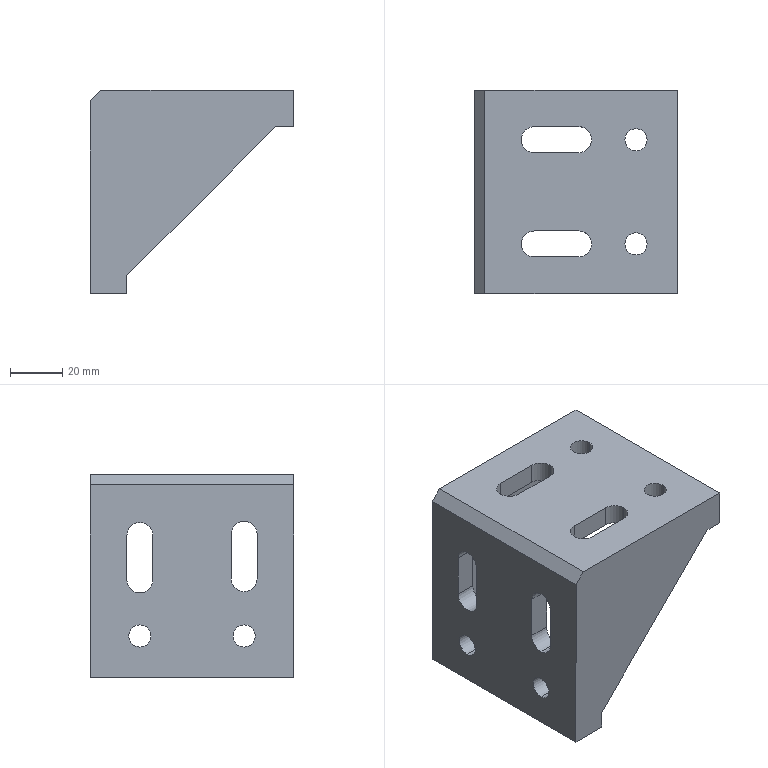Part | SolidWorks | features ICE 11, HoleWzd 2, Chamfer 1, Extrusion 1 | 1 solid | 45 faces | box 78 x 78 x 78 mm | volume 101387 mm3 | plane 25 | cylinder 20 | commonest cylinder face diameters 10 x12 8.5 x8
STEP:
#1=CARTESIAN_POINT('',(24.019,19.,55.578));
#2=VERTEX_POINT('',#1);
#3=CARTESIAN_POINT('',(32.519,19.,55.578));
#4=VERTEX_POINT('',#3);
#5=CARTESIAN_POINT('',(28.269,19.,55.578));
#6=DIRECTION('',(0.,0.,1.));
#7=DIRECTION('',(1.,0.,0.));
#8=AXIS2_PLACEMENT_3D('',#5,#6,#7);
#9=CIRCLE('',#8,4.25);
#10=EDGE_CURVE('',#2,#4,#9,.T.);
#11=ORIENTED_EDGE('',*,*,#10,.F.);
#12=CARTESIAN_POINT('',(24.019,19.,63.578));
#13=VERTEX_POINT('',#12);
#14=CARTESIAN_POINT('',(24.019,19.,63.578));
#15=DIRECTION('',(0.,0.,1.));
#16=VECTOR('',#15,1000.);
#17=LINE('',#14,#16);
#18=EDGE_CURVE('',#2,#13,#17,.T.);
#19=ORIENTED_EDGE('',*,*,#18,.T.);
#20=CARTESIAN_POINT('',(32.519,19.,63.578));
#21=VERTEX_POINT('',#20);
#22=CARTESIAN_POINT('',(28.269,19.,63.578));
#23=DIRECTION('',(0.,0.,1.));
#24=DIRECTION('',(1.,0.,0.));
#25=AXIS2_PLACEMENT_3D('',#22,#23,#24);
#26=CIRCLE('',#25,4.25);
#27=EDGE_CURVE('',#13,#21,#26,.T.);
#28=ORIENTED_EDGE('',*,*,#27,.T.);
#29=CARTESIAN_POINT('',(32.519,19.,63.578));
#30=DIRECTION('',(0.,0.,1.));
#31=VECTOR('',#30,1000.);
#32=LINE('',#29,#31);
#33=EDGE_CURVE('',#4,#21,#32,.T.);
#34=ORIENTED_EDGE('',*,*,#33,.F.);
#35=EDGE_LOOP('',(#11,#19,#28,#34));
#36=FACE_OUTER_BOUND('',#35,.T.);
#37=CARTESIAN_POINT('',(28.269,19.,63.578));
#38=DIRECTION('',(0.,0.,1.));
#39=DIRECTION('',(1.,0.,0.));
#40=AXIS2_PLACEMENT_3D('',#37,#38,#39);
#41=CYLINDRICAL_SURFACE('',#40,4.25);
#42=ADVANCED_FACE('',(#36),#41,.F.);
#43=CARTESIAN_POINT('',(24.019,59.,55.578));
#44=VERTEX_POINT('',#43);
#45=CARTESIAN_POINT('',(32.519,59.,55.578));
#46=VERTEX_POINT('',#45);
#47=CARTESIAN_POINT('',(28.269,59.,55.578));
#48=DIRECTION('',(0.,0.,1.));
#49=DIRECTION('',(1.,0.,0.));
#50=AXIS2_PLACEMENT_3D('',#47,#48,#49);
#51=CIRCLE('',#50,4.25);
#52=EDGE_CURVE('',#44,#46,#51,.T.);
#53=ORIENTED_EDGE('',*,*,#52,.F.);
#54=CARTESIAN_POINT('',(24.019,59.,63.578));
#55=VERTEX_POINT('',#54);
#56=CARTESIAN_POINT('',(24.019,59.,63.578));
#57=DIRECTION('',(0.,0.,1.));
#58=VECTOR('',#57,1000.);
#59=LINE('',#56,#58);
#60=EDGE_CURVE('',#44,#55,#59,.T.);
#61=ORIENTED_EDGE('',*,*,#60,.T.);
#62=CARTESIAN_POINT('',(32.519,59.,63.578));
#63=VERTEX_POINT('',#62);
#64=CARTESIAN_POINT('',(28.269,59.,63.578));
#65=DIRECTION('',(0.,0.,1.));
#66=DIRECTION('',(1.,0.,0.));
#67=AXIS2_PLACEMENT_3D('',#64,#65,#66);
#68=CIRCLE('',#67,4.25);
#69=EDGE_CURVE('',#55,#63,#68,.T.);
#70=ORIENTED_EDGE('',*,*,#69,.T.);
#71=CARTESIAN_POINT('',(32.519,59.,63.578));
#72=DIRECTION('',(0.,0.,1.));
#73=VECTOR('',#72,1000.);
#74=LINE('',#71,#73);
#75=EDGE_CURVE('',#46,#63,#74,.T.);
#76=ORIENTED_EDGE('',*,*,#75,.F.);
#77=EDGE_LOOP('',(#53,#61,#70,#76));
#78=FACE_OUTER_BOUND('',#77,.T.);
#79=CARTESIAN_POINT('',(28.269,59.,63.578));
#80=DIRECTION('',(0.,0.,1.));
#81=DIRECTION('',(1.,0.,0.));
#82=AXIS2_PLACEMENT_3D('',#79,#80,#81);
#83=CYLINDRICAL_SURFACE('',#82,4.25);
#84=ADVANCED_FACE('',(#78),#83,.F.);
#85=CARTESIAN_POINT('',(-25.731,59.,-2.672));
#86=VERTEX_POINT('',#85);
#87=CARTESIAN_POINT('',(-25.731,59.,5.828));
#88=VERTEX_POINT('',#87);
#89=CARTESIAN_POINT('',(-25.731,59.,1.578));
#90=DIRECTION('',(-1.,0.,0.));
#91=DIRECTION('',(0.,0.,1.));
#92=AXIS2_PLACEMENT_3D('',#89,#90,#91);
#93=CIRCLE('',#92,4.25);
#94=EDGE_CURVE('',#86,#88,#93,.T.);
#95=ORIENTED_EDGE('',*,*,#94,.F.);
#96=CARTESIAN_POINT('',(-33.731,59.,-2.672));
#97=VERTEX_POINT('',#96);
#98=CARTESIAN_POINT('',(-33.731,59.,-2.672));
#99=DIRECTION('',(-1.,0.,0.));
#100=VECTOR('',#99,1000.);
#101=LINE('',#98,#100);
#102=EDGE_CURVE('',#86,#97,#101,.T.);
#103=ORIENTED_EDGE('',*,*,#102,.T.);
#104=CARTESIAN_POINT('',(-33.731,59.,5.828));
#105=VERTEX_POINT('',#104);
#106=CARTESIAN_POINT('',(-33.731,59.,1.578));
#107=DIRECTION('',(-1.,0.,0.));
#108=DIRECTION('',(0.,0.,1.));
#109=AXIS2_PLACEMENT_3D('',#106,#107,#108);
#110=CIRCLE('',#109,4.25);
#111=EDGE_CURVE('',#97,#105,#110,.T.);
#112=ORIENTED_EDGE('',*,*,#111,.T.);
#113=CARTESIAN_POINT('',(-33.731,59.,5.828));
#114=DIRECTION('',(-1.,0.,0.));
#115=VECTOR('',#114,1000.);
#116=LINE('',#113,#115);
#117=EDGE_CURVE('',#88,#105,#116,.T.);
#118=ORIENTED_EDGE('',*,*,#117,.F.);
#119=EDGE_LOOP('',(#95,#103,#112,#118));
#120=FACE_OUTER_BOUND('',#119,.T.);
#121=CARTESIAN_POINT('',(-33.731,59.,1.578));
#122=DIRECTION('',(-1.,0.,0.));
#123=DIRECTION('',(0.,0.,1.));
#124=AXIS2_PLACEMENT_3D('',#121,#122,#123);
#125=CYLINDRICAL_SURFACE('',#124,4.25);
#126=ADVANCED_FACE('',(#120),#125,.F.);
#127=CARTESIAN_POINT('',(-25.731,19.,-2.672));
#128=VERTEX_POINT('',#127);
#129=CARTESIAN_POINT('',(-25.731,19.,5.828));
#130=VERTEX_POINT('',#129);
#131=CARTESIAN_POINT('',(-25.731,19.,1.578));
#132=DIRECTION('',(-1.,0.,0.));
#133=DIRECTION('',(0.,0.,1.));
#134=AXIS2_PLACEMENT_3D('',#131,#132,#133);
#135=CIRCLE('',#134,4.25);
#136=EDGE_CURVE('',#128,#130,#135,.T.);
#137=ORIENTED_EDGE('',*,*,#136,.F.);
#138=CARTESIAN_POINT('',(-33.731,19.,-2.672));
#139=VERTEX_POINT('',#138);
#140=CARTESIAN_POINT('',(-33.731,19.,-2.672));
#141=DIRECTION('',(-1.,0.,0.));
#142=VECTOR('',#141,1000.);
#143=LINE('',#140,#142);
#144=EDGE_CURVE('',#128,#139,#143,.T.);
#145=ORIENTED_EDGE('',*,*,#144,.T.);
#146=CARTESIAN_POINT('',(-33.731,19.,5.828));
#147=VERTEX_POINT('',#146);
#148=CARTESIAN_POINT('',(-33.731,19.,1.578));
#149=DIRECTION('',(-1.,0.,0.));
#150=DIRECTION('',(0.,0.,1.));
#151=AXIS2_PLACEMENT_3D('',#148,#149,#150);
#152=CIRCLE('',#151,4.25);
#153=EDGE_CURVE('',#139,#147,#152,.T.);
#154=ORIENTED_EDGE('',*,*,#153,.T.);
#155=CARTESIAN_POINT('',(-33.731,19.,5.828));
#156=DIRECTION('',(-1.,0.,0.));
#157=VECTOR('',#156,1000.);
#158=LINE('',#155,#157);
#159=EDGE_CURVE('',#130,#147,#158,.T.);
#160=ORIENTED_EDGE('',*,*,#159,.F.);
#161=EDGE_LOOP('',(#137,#145,#154,#160));
#162=FACE_OUTER_BOUND('',#161,.T.);
#163=CARTESIAN_POINT('',(-33.731,19.,1.578));
#164=DIRECTION('',(-1.,0.,0.));
#165=DIRECTION('',(0.,0.,1.));
#166=AXIS2_PLACEMENT_3D('',#163,#164,#165);
#167=CYLINDRICAL_SURFACE('',#166,4.25);
#168=ADVANCED_FACE('',(#162),#167,.F.);
#169=CARTESIAN_POINT('',(-25.731,59.,45.078));
#170=VERTEX_POINT('',#169);
#171=CARTESIAN_POINT('',(-25.731,64.,40.078));
#172=VERTEX_POINT('',#171);
#173=CARTESIAN_POINT('',(-25.731,59.,40.078));
#174=DIRECTION('',(-1.,0.,0.));
#175=DIRECTION('',(0.,0.,1.));
#176=AXIS2_PLACEMENT_3D('',#173,#174,#175);
#177=CIRCLE('',#176,5.);
#178=EDGE_CURVE('',#170,#172,#177,.T.);
#179=ORIENTED_EDGE('',*,*,#178,.F.);
#180=CARTESIAN_POINT('',(-33.731,59.,45.078));
#181=VERTEX_POINT('',#180);
#182=CARTESIAN_POINT('',(44.269,59.,45.078));
#183=DIRECTION('',(-1.,0.,0.));
#184=VECTOR('',#183,1000.);
#185=LINE('',#182,#184);
#186=EDGE_CURVE('',#170,#181,#185,.T.);
#187=ORIENTED_EDGE('',*,*,#186,.T.);
#188=CARTESIAN_POINT('',(-33.731,64.,40.078));
#189=VERTEX_POINT('',#188);
#190=CARTESIAN_POINT('',(-33.731,59.,40.078));
#191=DIRECTION('',(-1.,0.,0.));
#192=DIRECTION('',(0.,0.,1.));
#193=AXIS2_PLACEMENT_3D('',#190,#191,#192);
#194=CIRCLE('',#193,5.);
#195=EDGE_CURVE('',#181,#189,#194,.T.);
#196=ORIENTED_EDGE('',*,*,#195,.T.);
#197=CARTESIAN_POINT('',(44.269,64.,40.078));
#198=DIRECTION('',(-1.,0.,0.));
#199=VECTOR('',#198,1000.);
#200=LINE('',#197,#199);
#201=EDGE_CURVE('',#172,#189,#200,.T.);
#202=ORIENTED_EDGE('',*,*,#201,.F.);
#203=EDGE_LOOP('',(#179,#187,#196,#202));
#204=FACE_OUTER_BOUND('',#203,.T.);
#205=CARTESIAN_POINT('',(44.269,59.,40.078));
#206=DIRECTION('',(-1.,0.,0.));
#207=DIRECTION('',(0.,0.,1.));
#208=AXIS2_PLACEMENT_3D('',#205,#206,#207);
#209=CYLINDRICAL_SURFACE('',#208,5.);
#210=ADVANCED_FACE('',(#204),#209,.F.);
#211=CARTESIAN_POINT('',(11.269,19.,55.578));
#212=VERTEX_POINT('',#211);
#213=CARTESIAN_POINT('',(6.269,24.,55.578));
#214=VERTEX_POINT('',#213);
#215=CARTESIAN_POINT('',(6.269,19.,55.578));
#216=DIRECTION('',(0.,0.,1.));
#217=DIRECTION('',(1.,0.,0.));
#218=AXIS2_PLACEMENT_3D('',#215,#216,#217);
#219=CIRCLE('',#218,5.);
#220=EDGE_CURVE('',#212,#214,#219,.T.);
#221=ORIENTED_EDGE('',*,*,#220,.F.);
#222=CARTESIAN_POINT('',(11.269,19.,63.578));
#223=VERTEX_POINT('',#222);
#224=CARTESIAN_POINT('',(11.269,19.,-14.422));
#225=DIRECTION('',(0.,0.,1.));
#226=VECTOR('',#225,1000.);
#227=LINE('',#224,#226);
#228=EDGE_CURVE('',#212,#223,#227,.T.);
#229=ORIENTED_EDGE('',*,*,#228,.T.);
#230=CARTESIAN_POINT('',(6.269,24.,63.578));
#231=VERTEX_POINT('',#230);
#232=CARTESIAN_POINT('',(6.269,19.,63.578));
#233=DIRECTION('',(0.,0.,1.));
#234=DIRECTION('',(1.,0.,0.));
#235=AXIS2_PLACEMENT_3D('',#232,#233,#234);
#236=CIRCLE('',#235,5.);
#237=EDGE_CURVE('',#223,#231,#236,.T.);
#238=ORIENTED_EDGE('',*,*,#237,.T.);
#239=CARTESIAN_POINT('',(6.269,24.,-14.422));
#240=DIRECTION('',(0.,0.,1.));
#241=VECTOR('',#240,1000.);
#242=LINE('',#239,#241);
#243=EDGE_CURVE('',#214,#231,#242,.T.);
#244=ORIENTED_EDGE('',*,*,#243,.F.);
#245=EDGE_LOOP('',(#221,#229,#238,#244));
#246=FACE_OUTER_BOUND('',#245,.T.);
#247=CARTESIAN_POINT('',(6.269,19.,-14.422));
#248=DIRECTION('',(0.,0.,1.));
#249=DIRECTION('',(1.,0.,0.));
#250=AXIS2_PLACEMENT_3D('',#247,#248,#249);
#251=CYLINDRICAL_SURFACE('',#250,5.);
#252=ADVANCED_FACE('',(#246),#251,.F.);
#253=CARTESIAN_POINT('',(11.269,59.,55.578));
#254=VERTEX_POINT('',#253);
#255=CARTESIAN_POINT('',(6.269,64.,55.578));
#256=VERTEX_POINT('',#255);
#257=CARTESIAN_POINT('',(6.269,59.,55.578));
#258=DIRECTION('',(0.,0.,1.));
#259=DIRECTION('',(1.,0.,0.));
#260=AXIS2_PLACEMENT_3D('',#257,#258,#259);
#261=CIRCLE('',#260,5.);
#262=EDGE_CURVE('',#254,#256,#261,.T.);
#263=ORIENTED_EDGE('',*,*,#262,.F.);
#264=CARTESIAN_POINT('',(11.269,59.,63.578));
#265=VERTEX_POINT('',#264);
#266=CARTESIAN_POINT('',(11.269,59.,-14.422));
#267=DIRECTION('',(0.,0.,1.));
#268=VECTOR('',#267,1000.);
#269=LINE('',#266,#268);
#270=EDGE_CURVE('',#254,#265,#269,.T.);
#271=ORIENTED_EDGE('',*,*,#270,.T.);
#272=CARTESIAN_POINT('',(6.269,64.,63.578));
#273=VERTEX_POINT('',#272);
#274=CARTESIAN_POINT('',(6.269,59.,63.578));
#275=DIRECTION('',(0.,0.,1.));
#276=DIRECTION('',(1.,0.,0.));
#277=AXIS2_PLACEMENT_3D('',#274,#275,#276);
#278=CIRCLE('',#277,5.);
#279=EDGE_CURVE('',#265,#273,#278,.T.);
#280=ORIENTED_EDGE('',*,*,#279,.T.);
#281=CARTESIAN_POINT('',(6.269,64.,-14.422));
#282=DIRECTION('',(0.,0.,1.));
#283=VECTOR('',#282,1000.);
#284=LINE('',#281,#283);
#285=EDGE_CURVE('',#256,#273,#284,.T.);
#286=ORIENTED_EDGE('',*,*,#285,.F.);
#287=EDGE_LOOP('',(#263,#271,#280,#286));
#288=FACE_OUTER_BOUND('',#287,.T.);
#289=CARTESIAN_POINT('',(6.269,59.,-14.422));
#290=DIRECTION('',(0.,0.,1.));
#291=DIRECTION('',(1.,0.,0.));
#292=AXIS2_PLACEMENT_3D('',#289,#290,#291);
#293=CYLINDRICAL_SURFACE('',#292,5.);
#294=ADVANCED_FACE('',(#288),#293,.F.);
#295=CARTESIAN_POINT('',(-33.731,19.,18.578));
#296=VERTEX_POINT('',#295);
#297=CARTESIAN_POINT('',(-33.731,24.,23.578));
#298=VERTEX_POINT('',#297);
#299=CARTESIAN_POINT('',(-33.731,19.,23.578));
#300=DIRECTION('',(1.,0.,0.));
#301=DIRECTION('',(0.,0.,-1.));
#302=AXIS2_PLACEMENT_3D('',#299,#300,#301);
#303=CIRCLE('',#302,5.);
#304=EDGE_CURVE('',#296,#298,#303,.T.);
#305=ORIENTED_EDGE('',*,*,#304,.F.);
#306=CARTESIAN_POINT('',(-25.731,19.,18.578));
#307=VERTEX_POINT('',#306);
#308=CARTESIAN_POINT('',(-33.731,19.,18.578));
#309=DIRECTION('',(1.,0.,0.));
#310=VECTOR('',#309,1000.);
#311=LINE('',#308,#310);
#312=EDGE_CURVE('',#296,#307,#311,.T.);
#313=ORIENTED_EDGE('',*,*,#312,.T.);
#314=CARTESIAN_POINT('',(-25.731,24.,23.578));
#315=VERTEX_POINT('',#314);
#316=CARTESIAN_POINT('',(-25.731,19.,23.578));
#317=DIRECTION('',(1.,0.,0.));
#318=DIRECTION('',(0.,0.,-1.));
#319=AXIS2_PLACEMENT_3D('',#316,#317,#318);
#320=CIRCLE('',#319,5.);
#321=EDGE_CURVE('',#307,#315,#320,.T.);
#322=ORIENTED_EDGE('',*,*,#321,.T.);
#323=CARTESIAN_POINT('',(-33.731,24.,23.578));
#324=DIRECTION('',(1.,0.,0.));
#325=VECTOR('',#324,1000.);
#326=LINE('',#323,#325);
#327=EDGE_CURVE('',#298,#315,#326,.T.);
#328=ORIENTED_EDGE('',*,*,#327,.F.);
#329=EDGE_LOOP('',(#305,#313,#322,#328));
#330=FACE_OUTER_BOUND('',#329,.T.);
#331=CARTESIAN_POINT('',(-33.731,19.,23.578));
#332=DIRECTION('',(1.,0.,0.));
#333=DIRECTION('',(0.,0.,-1.));
#334=AXIS2_PLACEMENT_3D('',#331,#332,#333);
#335=CYLINDRICAL_SURFACE('',#334,5.);
#336=ADVANCED_FACE('',(#330),#335,.F.);
#337=CARTESIAN_POINT('',(-19.731,74.,-7.422));
#338=VERTEX_POINT('',#337);
#339=CARTESIAN_POINT('',(37.269,74.,49.578));
#340=VERTEX_POINT('',#339);
#341=CARTESIAN_POINT('',(-19.731,74.,-7.422));
#342=DIRECTION('',(0.7071,0.,0.7071));
#343=VECTOR('',#342,1000.);
#344=LINE('',#341,#343);
#345=EDGE_CURVE('',#338,#340,#344,.T.);
#346=ORIENTED_EDGE('',*,*,#345,.F.);
#347=CARTESIAN_POINT('',(-19.731,78.,-7.422));
#348=VERTEX_POINT('',#347);
#349=CARTESIAN_POINT('',(-19.731,4.,-7.422));
#350=DIRECTION('',(0.,1.,0.));
#351=VECTOR('',#350,1000.);
#352=LINE('',#349,#351);
#353=EDGE_CURVE('',#338,#348,#352,.T.);
#354=ORIENTED_EDGE('',*,*,#353,.T.);
#355=CARTESIAN_POINT('',(37.269,78.,49.578));
#356=VERTEX_POINT('',#355);
#357=CARTESIAN_POINT('',(37.269,78.,49.578));
#358=DIRECTION('',(-0.7071,0.,-0.7071));
#359=VECTOR('',#358,1000.);
#360=LINE('',#357,#359);
#361=EDGE_CURVE('',#356,#348,#360,.T.);
#362=ORIENTED_EDGE('',*,*,#361,.F.);
#363=CARTESIAN_POINT('',(37.269,4.,49.578));
#364=DIRECTION('',(0.,1.,0.));
#365=VECTOR('',#364,1000.);
#366=LINE('',#363,#365);
#367=EDGE_CURVE('',#340,#356,#366,.T.);
#368=ORIENTED_EDGE('',*,*,#367,.F.);
#369=EDGE_LOOP('',(#346,#354,#362,#368));
#370=FACE_OUTER_BOUND('',#369,.T.);
#371=CARTESIAN_POINT('',(37.269,4.,49.578));
#372=DIRECTION('',(0.7071,0.,-0.7071));
#373=DIRECTION('',(-0.7071,0.,-0.7071));
#374=AXIS2_PLACEMENT_3D('',#371,#372,#373);
#375=PLANE('',#374);
#376=ADVANCED_FACE('',(#370),#375,.T.);
#377=CARTESIAN_POINT('',(-33.731,78.,59.578));
#378=VERTEX_POINT('',#377);
#379=CARTESIAN_POINT('',(-33.731,78.,-14.422));
#380=VERTEX_POINT('',#379);
#381=CARTESIAN_POINT('',(-33.731,78.,-14.422));
#382=DIRECTION('',(0.,0.,-1.));
#383=VECTOR('',#382,1000.);
#384=LINE('',#381,#383);
#385=EDGE_CURVE('',#378,#380,#384,.T.);
#386=ORIENTED_EDGE('',*,*,#385,.F.);
#387=CARTESIAN_POINT('',(-29.731,78.,63.578));
#388=VERTEX_POINT('',#387);
#389=CARTESIAN_POINT('',(-46.655,78.,46.655));
#390=DIRECTION('',(0.7071,0.,0.7071));
#391=VECTOR('',#390,1000.);
#392=LINE('',#389,#391);
#393=EDGE_CURVE('',#378,#388,#392,.T.);
#394=ORIENTED_EDGE('',*,*,#393,.T.);
#395=CARTESIAN_POINT('',(44.269,78.,63.578));
#396=VERTEX_POINT('',#395);
#397=CARTESIAN_POINT('',(-19.731,78.,63.578));
#398=DIRECTION('',(-1.,0.,0.));
#399=VECTOR('',#398,1000.);
#400=LINE('',#397,#399);
#401=EDGE_CURVE('',#396,#388,#400,.T.);
#402=ORIENTED_EDGE('',*,*,#401,.F.);
#403=CARTESIAN_POINT('',(44.269,78.,49.578));
#404=VERTEX_POINT('',#403);
#405=CARTESIAN_POINT('',(44.269,78.,63.578));
#406=DIRECTION('',(0.,0.,-1.));
#407=VECTOR('',#406,1000.);
#408=LINE('',#405,#407);
#409=EDGE_CURVE('',#396,#404,#408,.T.);
#410=ORIENTED_EDGE('',*,*,#409,.T.);
#411=CARTESIAN_POINT('',(-19.731,78.,49.578));
#412=DIRECTION('',(-1.,0.,0.));
#413=VECTOR('',#412,1000.);
#414=LINE('',#411,#413);
#415=EDGE_CURVE('',#404,#356,#414,.T.);
#416=ORIENTED_EDGE('',*,*,#415,.T.);
#417=ORIENTED_EDGE('',*,*,#361,.T.);
#418=CARTESIAN_POINT('',(-19.731,78.,-14.422));
#419=VERTEX_POINT('',#418);
#420=CARTESIAN_POINT('',(-19.731,78.,-14.422));
#421=DIRECTION('',(0.,0.,-1.));
#422=VECTOR('',#421,1000.);
#423=LINE('',#420,#422);
#424=EDGE_CURVE('',#348,#419,#423,.T.);
#425=ORIENTED_EDGE('',*,*,#424,.T.);
#426=CARTESIAN_POINT('',(-33.731,78.,-14.422));
#427=DIRECTION('',(1.,0.,0.));
#428=VECTOR('',#427,1000.);
#429=LINE('',#426,#428);
#430=EDGE_CURVE('',#380,#419,#429,.T.);
#431=ORIENTED_EDGE('',*,*,#430,.F.);
#432=EDGE_LOOP('',(#386,#394,#402,#410,#416,#417,#425,#431));
#433=FACE_OUTER_BOUND('',#432,.T.);
#434=CARTESIAN_POINT('',(0.,78.,0.));
#435=DIRECTION('',(0.,1.,0.));
#436=DIRECTION('',(0.,0.,1.));
#437=AXIS2_PLACEMENT_3D('',#434,#435,#436);
#438=PLANE('',#437);
#439=ADVANCED_FACE('',(#433),#438,.T.);
#440=CARTESIAN_POINT('',(44.269,0.,49.578));
#441=VERTEX_POINT('',#440);
#442=CARTESIAN_POINT('',(44.269,0.,63.578));
#443=VERTEX_POINT('',#442);
#444=CARTESIAN_POINT('',(44.269,0.,63.578));
#445=DIRECTION('',(0.,0.,1.));
#446=VECTOR('',#445,1000.);
#447=LINE('',#444,#446);
#448=EDGE_CURVE('',#441,#443,#447,.T.);
#449=ORIENTED_EDGE('',*,*,#448,.F.);
#450=CARTESIAN_POINT('',(44.269,4.,49.578));
#451=VERTEX_POINT('',#450);
#452=CARTESIAN_POINT('',(44.269,78.,49.578));
#453=DIRECTION('',(0.,-1.,0.));
#454=VECTOR('',#453,1000.);
#455=LINE('',#452,#454);
#456=EDGE_CURVE('',#451,#441,#455,.T.);
#457=ORIENTED_EDGE('',*,*,#456,.F.);
#458=CARTESIAN_POINT('',(44.269,4.,55.578));
#459=VERTEX_POINT('',#458);
#460=CARTESIAN_POINT('',(44.269,4.,63.578));
#461=DIRECTION('',(0.,0.,1.));
#462=VECTOR('',#461,1000.);
#463=LINE('',#460,#462);
#464=EDGE_CURVE('',#451,#459,#463,.T.);
#465=ORIENTED_EDGE('',*,*,#464,.T.);
#466=CARTESIAN_POINT('',(44.269,74.,55.578));
#467=VERTEX_POINT('',#466);
#468=CARTESIAN_POINT('',(44.269,4.,55.578));
#469=DIRECTION('',(0.,1.,0.));
#470=VECTOR('',#469,1000.);
#471=LINE('',#468,#470);
#472=EDGE_CURVE('',#459,#467,#471,.T.);
#473=ORIENTED_EDGE('',*,*,#472,.T.);
#474=CARTESIAN_POINT('',(44.269,74.,49.578));
#475=VERTEX_POINT('',#474);
#476=CARTESIAN_POINT('',(44.269,74.,-45.269));
#477=DIRECTION('',(0.,0.,1.));
#478=VECTOR('',#477,1000.);
#479=LINE('',#476,#478);
#480=EDGE_CURVE('',#475,#467,#479,.T.);
#481=ORIENTED_EDGE('',*,*,#480,.F.);
#482=CARTESIAN_POINT('',(44.269,78.,49.578));
#483=DIRECTION('',(0.,1.,0.));
#484=VECTOR('',#483,1000.);
#485=LINE('',#482,#484);
#486=EDGE_CURVE('',#475,#404,#485,.T.);
#487=ORIENTED_EDGE('',*,*,#486,.T.);
#488=ORIENTED_EDGE('',*,*,#409,.F.);
#489=CARTESIAN_POINT('',(44.269,78.,63.578));
#490=DIRECTION('',(0.,1.,0.));
#491=VECTOR('',#490,1000.);
#492=LINE('',#489,#491);
#493=EDGE_CURVE('',#443,#396,#492,.T.);
#494=ORIENTED_EDGE('',*,*,#493,.F.);
#495=EDGE_LOOP('',(#449,#457,#465,#473,#481,#487,#488,#494));
#496=FACE_OUTER_BOUND('',#495,.T.);
#497=CARTESIAN_POINT('',(44.269,78.,63.578));
#498=DIRECTION('',(-1.,0.,0.));
#499=DIRECTION('',(0.,0.,1.));
#500=AXIS2_PLACEMENT_3D('',#497,#498,#499);
#501=PLANE('',#500);
#502=ADVANCED_FACE('',(#496),#501,.F.);
#503=CARTESIAN_POINT('',(28.269,19.,63.578));
#504=DIRECTION('',(0.,0.,1.));
#505=DIRECTION('',(1.,0.,0.));
#506=AXIS2_PLACEMENT_3D('',#503,#504,#505);
#507=CIRCLE('',#506,4.25);
#508=EDGE_CURVE('',#21,#13,#507,.T.);
#509=ORIENTED_EDGE('',*,*,#508,.F.);
#510=ORIENTED_EDGE('',*,*,#27,.F.);
#511=EDGE_LOOP('',(#509,#510));
#512=FACE_BOUND('',#511,.T.);
#513=CARTESIAN_POINT('',(28.269,59.,63.578));
#514=DIRECTION('',(0.,0.,1.));
#515=DIRECTION('',(1.,0.,0.));
#516=AXIS2_PLACEMENT_3D('',#513,#514,#515);
#517=CIRCLE('',#516,4.25);
#518=EDGE_CURVE('',#63,#55,#517,.T.);
#519=ORIENTED_EDGE('',*,*,#518,.F.);
#520=ORIENTED_EDGE('',*,*,#69,.F.);
#521=EDGE_LOOP('',(#519,#520));
#522=FACE_BOUND('',#521,.T.);
#523=CARTESIAN_POINT('',(-10.731,24.,63.578));
#524=VERTEX_POINT('',#523);
#525=CARTESIAN_POINT('',(6.269,24.,63.578));
#526=DIRECTION('',(-1.,0.,0.));
#527=VECTOR('',#526,1000.);
#528=LINE('',#525,#527);
#529=EDGE_CURVE('',#231,#524,#528,.T.);
#530=ORIENTED_EDGE('',*,*,#529,.F.);
#531=ORIENTED_EDGE('',*,*,#237,.F.);
#532=CARTESIAN_POINT('',(6.269,14.,63.578));
#533=VERTEX_POINT('',#532);
#534=CARTESIAN_POINT('',(6.269,19.,63.578));
#535=DIRECTION('',(0.,0.,1.));
#536=DIRECTION('',(1.,0.,0.));
#537=AXIS2_PLACEMENT_3D('',#534,#535,#536);
#538=CIRCLE('',#537,5.);
#539=EDGE_CURVE('',#533,#223,#538,.T.);
#540=ORIENTED_EDGE('',*,*,#539,.F.);
#541=CARTESIAN_POINT('',(-10.731,14.,63.578));
#542=VERTEX_POINT('',#541);
#543=CARTESIAN_POINT('',(-10.731,14.,63.578));
#544=DIRECTION('',(1.,0.,0.));
#545=VECTOR('',#544,1000.);
#546=LINE('',#543,#545);
#547=EDGE_CURVE('',#542,#533,#546,.T.);
#548=ORIENTED_EDGE('',*,*,#547,.F.);
#549=CARTESIAN_POINT('',(-10.731,19.,63.578));
#550=DIRECTION('',(0.,0.,1.));
#551=DIRECTION('',(1.,0.,0.));
#552=AXIS2_PLACEMENT_3D('',#549,#550,#551);
#553=CIRCLE('',#552,5.);
#554=EDGE_CURVE('',#524,#542,#553,.T.);
#555=ORIENTED_EDGE('',*,*,#554,.F.);
#556=EDGE_LOOP('',(#530,#531,#540,#548,#555));
#557=FACE_BOUND('',#556,.T.);
#558=CARTESIAN_POINT('',(-10.731,64.,63.578));
#559=VERTEX_POINT('',#558);
#560=CARTESIAN_POINT('',(6.269,64.,63.578));
#561=DIRECTION('',(-1.,0.,0.));
#562=VECTOR('',#561,1000.);
#563=LINE('',#560,#562);
#564=EDGE_CURVE('',#273,#559,#563,.T.);
#565=ORIENTED_EDGE('',*,*,#564,.F.);
#566=ORIENTED_EDGE('',*,*,#279,.F.);
#567=CARTESIAN_POINT('',(6.269,54.,63.578));
#568=VERTEX_POINT('',#567);
#569=CARTESIAN_POINT('',(6.269,59.,63.578));
#570=DIRECTION('',(0.,0.,1.));
#571=DIRECTION('',(1.,0.,0.));
#572=AXIS2_PLACEMENT_3D('',#569,#570,#571);
#573=CIRCLE('',#572,5.);
#574=EDGE_CURVE('',#568,#265,#573,.T.);
#575=ORIENTED_EDGE('',*,*,#574,.F.);
#576=CARTESIAN_POINT('',(-10.731,54.,63.578));
#577=VERTEX_POINT('',#576);
#578=CARTESIAN_POINT('',(-10.731,54.,63.578));
#579=DIRECTION('',(1.,0.,0.));
#580=VECTOR('',#579,1000.);
#581=LINE('',#578,#580);
#582=EDGE_CURVE('',#577,#568,#581,.T.);
#583=ORIENTED_EDGE('',*,*,#582,.F.);
#584=CARTESIAN_POINT('',(-10.731,59.,63.578));
#585=DIRECTION('',(0.,0.,1.));
#586=DIRECTION('',(1.,0.,0.));
#587=AXIS2_PLACEMENT_3D('',#584,#585,#586);
#588=CIRCLE('',#587,5.);
#589=EDGE_CURVE('',#559,#577,#588,.T.);
#590=ORIENTED_EDGE('',*,*,#589,.F.);
#591=EDGE_LOOP('',(#565,#566,#575,#583,#590));
#592=FACE_BOUND('',#591,.T.);
#593=ORIENTED_EDGE('',*,*,#401,.T.);
#594=CARTESIAN_POINT('',(-29.731,0.,63.578));
#595=VERTEX_POINT('',#594);
#596=CARTESIAN_POINT('',(-29.731,0.,63.578));
#597=DIRECTION('',(0.,-1.,0.));
#598=VECTOR('',#597,1000.);
#599=LINE('',#596,#598);
#600=EDGE_CURVE('',#388,#595,#599,.T.);
#601=ORIENTED_EDGE('',*,*,#600,.T.);
#602=CARTESIAN_POINT('',(-19.731,0.,63.578));
#603=DIRECTION('',(-1.,0.,0.));
#604=VECTOR('',#603,1000.);
#605=LINE('',#602,#604);
#606=EDGE_CURVE('',#443,#595,#605,.T.);
#607=ORIENTED_EDGE('',*,*,#606,.F.);
#608=ORIENTED_EDGE('',*,*,#493,.T.);
#609=EDGE_LOOP('',(#593,#601,#607,#608));
#610=FACE_OUTER_BOUND('',#609,.T.);
#611=CARTESIAN_POINT('',(0.,0.,63.578));
#612=DIRECTION('',(0.,0.,-1.));
#613=DIRECTION('',(-1.,0.,0.));
#614=AXIS2_PLACEMENT_3D('',#611,#612,#613);
#615=PLANE('',#614);
#616=ADVANCED_FACE('',(#512,#522,#557,#592,#610),#615,.F.);
#617=CARTESIAN_POINT('',(44.269,74.,49.578));
#618=DIRECTION('',(-1.,0.,0.));
#619=VECTOR('',#618,1000.);
#620=LINE('',#617,#619);
#621=EDGE_CURVE('',#475,#340,#620,.T.);
#622=ORIENTED_EDGE('',*,*,#621,.T.);
#623=ORIENTED_EDGE('',*,*,#367,.T.);
#624=ORIENTED_EDGE('',*,*,#415,.F.);
#625=ORIENTED_EDGE('',*,*,#486,.F.);
#626=EDGE_LOOP('',(#622,#623,#624,#625));
#627=FACE_OUTER_BOUND('',#626,.T.);
#628=CARTESIAN_POINT('',(0.,0.,49.578));
#629=DIRECTION('',(0.,0.,-1.));
#630=DIRECTION('',(-1.,0.,0.));
#631=AXIS2_PLACEMENT_3D('',#628,#629,#630);
#632=PLANE('',#631);
#633=ADVANCED_FACE('',(#627),#632,.T.);
#634=CARTESIAN_POINT('',(-19.731,4.,-14.422));
#635=VERTEX_POINT('',#634);
#636=CARTESIAN_POINT('',(-19.731,4.,-7.422));
#637=VERTEX_POINT('',#636);
#638=CARTESIAN_POINT('',(-19.731,4.,0.));
#639=DIRECTION('',(0.,0.,1.));
#640=VECTOR('',#639,1000.);
#641=LINE('',#638,#640);
#642=EDGE_CURVE('',#635,#637,#641,.T.);
#643=ORIENTED_EDGE('',*,*,#642,.F.);
#644=CARTESIAN_POINT('',(-25.731,4.,-14.422));
#645=VERTEX_POINT('',#644);
#646=CARTESIAN_POINT('',(44.269,4.,-14.422));
#647=DIRECTION('',(1.,0.,0.));
#648=VECTOR('',#647,1000.);
#649=LINE('',#646,#648);
#650=EDGE_CURVE('',#645,#635,#649,.T.);
#651=ORIENTED_EDGE('',*,*,#650,.F.);
#652=CARTESIAN_POINT('',(-25.731,4.,55.578));
#653=VERTEX_POINT('',#652);
#654=CARTESIAN_POINT('',(-25.731,4.,-14.422));
#655=DIRECTION('',(0.,0.,1.));
#656=VECTOR('',#655,1000.);
#657=LINE('',#654,#656);
#658=EDGE_CURVE('',#645,#653,#657,.T.);
#659=ORIENTED_EDGE('',*,*,#658,.T.);
#660=CARTESIAN_POINT('',(-19.731,4.,55.578));
#661=DIRECTION('',(1.,0.,0.));
#662=VECTOR('',#661,1000.);
#663=LINE('',#660,#662);
#664=EDGE_CURVE('',#653,#459,#663,.T.);
#665=ORIENTED_EDGE('',*,*,#664,.T.);
#666=ORIENTED_EDGE('',*,*,#464,.F.);
#667=CARTESIAN_POINT('',(37.269,4.,49.578));
#668=VERTEX_POINT('',#667);
#669=CARTESIAN_POINT('',(0.,4.,49.578));
#670=DIRECTION('',(1.,0.,0.));
#671=VECTOR('',#670,1000.);
#672=LINE('',#669,#671);
#673=EDGE_CURVE('',#668,#451,#672,.T.);
#674=ORIENTED_EDGE('',*,*,#673,.F.);
#675=CARTESIAN_POINT('',(-6.155,4.,6.155));
#676=DIRECTION('',(0.7071,0.,0.7071));
#677=VECTOR('',#676,1000.);
#678=LINE('',#675,#677);
#679=EDGE_CURVE('',#637,#668,#678,.T.);
#680=ORIENTED_EDGE('',*,*,#679,.F.);
#681=EDGE_LOOP('',(#643,#651,#659,#665,#666,#674,#680));
#682=FACE_OUTER_BOUND('',#681,.T.);
#683=CARTESIAN_POINT('',(0.,4.,0.));
#684=DIRECTION('',(0.,1.,0.));
#685=DIRECTION('',(0.,0.,1.));
#686=AXIS2_PLACEMENT_3D('',#683,#684,#685);
#687=PLANE('',#686);
#688=ADVANCED_FACE('',(#682),#687,.T.);
#689=ORIENTED_EDGE('',*,*,#650,.T.);
#690=CARTESIAN_POINT('',(-19.731,0.,-14.422));
#691=VERTEX_POINT('',#690);
#692=CARTESIAN_POINT('',(-19.731,78.,-14.422));
#693=DIRECTION('',(0.,-1.,0.));
#694=VECTOR('',#693,1000.);
#695=LINE('',#692,#694);
#696=EDGE_CURVE('',#635,#691,#695,.T.);
#697=ORIENTED_EDGE('',*,*,#696,.T.);
#698=CARTESIAN_POINT('',(-33.731,0.,-14.422));
#699=VERTEX_POINT('',#698);
#700=CARTESIAN_POINT('',(44.269,0.,-14.422));
#701=DIRECTION('',(1.,0.,0.));
#702=VECTOR('',#701,1000.);
#703=LINE('',#700,#702);
#704=EDGE_CURVE('',#699,#691,#703,.T.);
#705=ORIENTED_EDGE('',*,*,#704,.F.);
#706=CARTESIAN_POINT('',(-33.731,0.,-14.422));
#707=DIRECTION('',(0.,-1.,0.));
#708=VECTOR('',#707,1000.);
#709=LINE('',#706,#708);
#710=EDGE_CURVE('',#380,#699,#709,.T.);
#711=ORIENTED_EDGE('',*,*,#710,.F.);
#712=ORIENTED_EDGE('',*,*,#430,.T.);
#713=CARTESIAN_POINT('',(-19.731,74.,-14.422));
#714=VERTEX_POINT('',#713);
#715=CARTESIAN_POINT('',(-19.731,0.,-14.422));
#716=DIRECTION('',(0.,-1.,0.));
#717=VECTOR('',#716,1000.);
#718=LINE('',#715,#717);
#719=EDGE_CURVE('',#419,#714,#718,.T.);
#720=ORIENTED_EDGE('',*,*,#719,.T.);
#721=CARTESIAN_POINT('',(-25.731,74.,-14.422));
#722=VERTEX_POINT('',#721);
#723=CARTESIAN_POINT('',(79.264,74.,-14.422));
#724=DIRECTION('',(-1.,0.,0.));
#725=VECTOR('',#724,1000.);
#726=LINE('',#723,#725);
#727=EDGE_CURVE('',#714,#722,#726,.T.);
#728=ORIENTED_EDGE('',*,*,#727,.T.);
#729=CARTESIAN_POINT('',(-25.731,74.,-14.422));
#730=DIRECTION('',(0.,-1.,0.));
#731=VECTOR('',#730,1000.);
#732=LINE('',#729,#731);
#733=EDGE_CURVE('',#722,#645,#732,.T.);
#734=ORIENTED_EDGE('',*,*,#733,.T.);
#735=EDGE_LOOP('',(#689,#697,#705,#711,#712,#720,#728,#734));
#736=FACE_OUTER_BOUND('',#735,.T.);
#737=CARTESIAN_POINT('',(44.269,0.,-14.422));
#738=DIRECTION('',(0.,0.,1.));
#739=DIRECTION('',(1.,0.,0.));
#740=AXIS2_PLACEMENT_3D('',#737,#738,#739);
#741=PLANE('',#740);
#742=ADVANCED_FACE('',(#736),#741,.F.);
#743=ORIENTED_EDGE('',*,*,#606,.T.);
#744=CARTESIAN_POINT('',(-33.731,0.,59.578));
#745=VERTEX_POINT('',#744);
#746=CARTESIAN_POINT('',(-33.731,0.,59.578));
#747=DIRECTION('',(-0.7071,0.,-0.7071));
#748=VECTOR('',#747,1000.);
#749=LINE('',#746,#748);
#750=EDGE_CURVE('',#595,#745,#749,.T.);
#751=ORIENTED_EDGE('',*,*,#750,.T.);
#752=CARTESIAN_POINT('',(-33.731,0.,63.578));
#753=DIRECTION('',(0.,0.,1.));
#754=VECTOR('',#753,1000.);
#755=LINE('',#752,#754);
#756=EDGE_CURVE('',#699,#745,#755,.T.);
#757=ORIENTED_EDGE('',*,*,#756,.F.);
#758=ORIENTED_EDGE('',*,*,#704,.T.);
#759=CARTESIAN_POINT('',(-19.731,0.,-7.422));
#760=VERTEX_POINT('',#759);
#761=CARTESIAN_POINT('',(-19.731,0.,-7.422));
#762=DIRECTION('',(0.,0.,-1.));
#763=VECTOR('',#762,1000.);
#764=LINE('',#761,#763);
#765=EDGE_CURVE('',#760,#691,#764,.T.);
#766=ORIENTED_EDGE('',*,*,#765,.F.);
#767=CARTESIAN_POINT('',(37.269,0.,49.578));
#768=VERTEX_POINT('',#767);
#769=CARTESIAN_POINT('',(37.269,0.,49.578));
#770=DIRECTION('',(-0.7071,0.,-0.7071));
#771=VECTOR('',#770,1000.);
#772=LINE('',#769,#771);
#773=EDGE_CURVE('',#768,#760,#772,.T.);
#774=ORIENTED_EDGE('',*,*,#773,.F.);
#775=CARTESIAN_POINT('',(44.269,0.,49.578));
#776=DIRECTION('',(-1.,0.,0.));
#777=VECTOR('',#776,1000.);
#778=LINE('',#775,#777);
#779=EDGE_CURVE('',#441,#768,#778,.T.);
#780=ORIENTED_EDGE('',*,*,#779,.F.);
#781=ORIENTED_EDGE('',*,*,#448,.T.);
#782=EDGE_LOOP('',(#743,#751,#757,#758,#766,#774,#780,#781));
#783=FACE_OUTER_BOUND('',#782,.T.);
#784=CARTESIAN_POINT('',(0.,0.,0.));
#785=DIRECTION('',(0.,1.,0.));
#786=DIRECTION('',(0.,0.,1.));
#787=AXIS2_PLACEMENT_3D('',#784,#785,#786);
#788=PLANE('',#787);
#789=ADVANCED_FACE('',(#783),#788,.F.);
#790=CARTESIAN_POINT('',(-25.731,74.,55.578));
#791=VERTEX_POINT('',#790);
#792=CARTESIAN_POINT('',(44.269,74.,55.578));
#793=DIRECTION('',(-1.,0.,0.));
#794=VECTOR('',#793,1000.);
#795=LINE('',#792,#794);
#796=EDGE_CURVE('',#467,#791,#795,.T.);
#797=ORIENTED_EDGE('',*,*,#796,.T.);
#798=CARTESIAN_POINT('',(-25.731,74.,55.578));
#799=DIRECTION('',(0.,0.,-1.));
#800=VECTOR('',#799,1000.);
#801=LINE('',#798,#800);
#802=EDGE_CURVE('',#791,#722,#801,.T.);
#803=ORIENTED_EDGE('',*,*,#802,.T.);
#804=ORIENTED_EDGE('',*,*,#727,.F.);
#805=CARTESIAN_POINT('',(-19.731,74.,55.578));
#806=DIRECTION('',(0.,0.,-1.));
#807=VECTOR('',#806,1000.);
#808=LINE('',#805,#807);
#809=EDGE_CURVE('',#338,#714,#808,.T.);
#810=ORIENTED_EDGE('',*,*,#809,.F.);
#811=ORIENTED_EDGE('',*,*,#345,.T.);
#812=ORIENTED_EDGE('',*,*,#621,.F.);
#813=ORIENTED_EDGE('',*,*,#480,.T.);
#814=EDGE_LOOP('',(#797,#803,#804,#810,#811,#812,#813));
#815=FACE_OUTER_BOUND('',#814,.T.);
#816=CARTESIAN_POINT('',(0.,74.,0.));
#817=DIRECTION('',(0.,1.,0.));
#818=DIRECTION('',(0.,0.,1.));
#819=AXIS2_PLACEMENT_3D('',#816,#817,#818);
#820=PLANE('',#819);
#821=ADVANCED_FACE('',(#815),#820,.F.);
#822=CARTESIAN_POINT('',(-33.731,59.,1.578));
#823=DIRECTION('',(-1.,0.,0.));
#824=DIRECTION('',(0.,0.,1.));
#825=AXIS2_PLACEMENT_3D('',#822,#823,#824);
#826=CIRCLE('',#825,4.25);
#827=EDGE_CURVE('',#105,#97,#826,.T.);
#828=ORIENTED_EDGE('',*,*,#827,.F.);
#829=ORIENTED_EDGE('',*,*,#111,.F.);
#830=EDGE_LOOP('',(#828,#829));
#831=FACE_BOUND('',#830,.T.);
#832=CARTESIAN_POINT('',(-33.731,19.,1.578));
#833=DIRECTION('',(-1.,0.,0.));
#834=DIRECTION('',(0.,0.,1.));
#835=AXIS2_PLACEMENT_3D('',#832,#833,#834);
#836=CIRCLE('',#835,4.25);
#837=EDGE_CURVE('',#147,#139,#836,.T.);
#838=ORIENTED_EDGE('',*,*,#837,.F.);
#839=ORIENTED_EDGE('',*,*,#153,.F.);
#840=EDGE_LOOP('',(#838,#839));
#841=FACE_BOUND('',#840,.T.);
#842=CARTESIAN_POINT('',(-33.731,54.,23.078));
#843=VERTEX_POINT('',#842);
#844=CARTESIAN_POINT('',(-33.731,54.,40.078));
#845=VERTEX_POINT('',#844);
#846=CARTESIAN_POINT('',(-33.731,54.,23.078));
#847=DIRECTION('',(0.,0.,1.));
#848=VECTOR('',#847,1000.);
#849=LINE('',#846,#848);
#850=EDGE_CURVE('',#843,#845,#849,.T.);
#851=ORIENTED_EDGE('',*,*,#850,.F.);
#852=CARTESIAN_POINT('',(-33.731,64.,23.078));
#853=VERTEX_POINT('',#852);
#854=CARTESIAN_POINT('',(-33.731,59.,23.078));
#855=DIRECTION('',(-1.,0.,0.));
#856=DIRECTION('',(0.,0.,1.));
#857=AXIS2_PLACEMENT_3D('',#854,#855,#856);
#858=CIRCLE('',#857,5.);
#859=EDGE_CURVE('',#853,#843,#858,.T.);
#860=ORIENTED_EDGE('',*,*,#859,.F.);
#861=CARTESIAN_POINT('',(-33.731,64.,40.078));
#862=DIRECTION('',(0.,0.,-1.));
#863=VECTOR('',#862,1000.);
#864=LINE('',#861,#863);
#865=EDGE_CURVE('',#189,#853,#864,.T.);
#866=ORIENTED_EDGE('',*,*,#865,.F.);
#867=ORIENTED_EDGE('',*,*,#195,.F.);
#868=CARTESIAN_POINT('',(-33.731,59.,40.078));
#869=DIRECTION('',(-1.,0.,0.));
#870=DIRECTION('',(0.,0.,1.));
#871=AXIS2_PLACEMENT_3D('',#868,#869,#870);
#872=CIRCLE('',#871,5.);
#873=EDGE_CURVE('',#845,#181,#872,.T.);
#874=ORIENTED_EDGE('',*,*,#873,.F.);
#875=EDGE_LOOP('',(#851,#860,#866,#867,#874));
#876=FACE_BOUND('',#875,.T.);
#877=CARTESIAN_POINT('',(-33.731,14.,40.578));
#878=VERTEX_POINT('',#877);
#879=CARTESIAN_POINT('',(-33.731,14.,23.578));
#880=VERTEX_POINT('',#879);
#881=CARTESIAN_POINT('',(-33.731,14.,40.578));
#882=DIRECTION('',(0.,0.,-1.));
#883=VECTOR('',#882,1000.);
#884=LINE('',#881,#883);
#885=EDGE_CURVE('',#878,#880,#884,.T.);
#886=ORIENTED_EDGE('',*,*,#885,.T.);
#887=CARTESIAN_POINT('',(-33.731,19.,23.578));
#888=DIRECTION('',(1.,0.,0.));
#889=DIRECTION('',(0.,0.,-1.));
#890=AXIS2_PLACEMENT_3D('',#887,#888,#889);
#891=CIRCLE('',#890,5.);
#892=EDGE_CURVE('',#880,#296,#891,.T.);
#893=ORIENTED_EDGE('',*,*,#892,.T.);
#894=ORIENTED_EDGE('',*,*,#304,.T.);
#895=CARTESIAN_POINT('',(-33.731,24.,40.578));
#896=VERTEX_POINT('',#895);
#897=CARTESIAN_POINT('',(-33.731,24.,23.578));
#898=DIRECTION('',(0.,0.,1.));
#899=VECTOR('',#898,1000.);
#900=LINE('',#897,#899);
#901=EDGE_CURVE('',#298,#896,#900,.T.);
#902=ORIENTED_EDGE('',*,*,#901,.T.);
#903=CARTESIAN_POINT('',(-33.731,19.,40.578));
#904=DIRECTION('',(1.,0.,0.));
#905=DIRECTION('',(0.,0.,-1.));
#906=AXIS2_PLACEMENT_3D('',#903,#904,#905);
#907=CIRCLE('',#906,5.);
#908=EDGE_CURVE('',#896,#878,#907,.T.);
#909=ORIENTED_EDGE('',*,*,#908,.T.);
#910=EDGE_LOOP('',(#886,#893,#894,#902,#909));
#911=FACE_BOUND('',#910,.T.);
#912=ORIENTED_EDGE('',*,*,#756,.T.);
#913=CARTESIAN_POINT('',(-33.731,0.,59.578));
#914=DIRECTION('',(0.,1.,0.));
#915=VECTOR('',#914,1000.);
#916=LINE('',#913,#915);
#917=EDGE_CURVE('',#745,#378,#916,.T.);
#918=ORIENTED_EDGE('',*,*,#917,.T.);
#919=ORIENTED_EDGE('',*,*,#385,.T.);
#920=ORIENTED_EDGE('',*,*,#710,.T.);
#921=EDGE_LOOP('',(#912,#918,#919,#920));
#922=FACE_OUTER_BOUND('',#921,.T.);
#923=CARTESIAN_POINT('',(-33.731,0.,0.));
#924=DIRECTION('',(1.,0.,0.));
#925=DIRECTION('',(0.,0.,-1.));
#926=AXIS2_PLACEMENT_3D('',#923,#924,#925);
#927=PLANE('',#926);
#928=ADVANCED_FACE('',(#831,#841,#876,#911,#922),#927,.F.);
#929=ORIENTED_EDGE('',*,*,#809,.T.);
#930=ORIENTED_EDGE('',*,*,#719,.F.);
#931=ORIENTED_EDGE('',*,*,#424,.F.);
#932=ORIENTED_EDGE('',*,*,#353,.F.);
#933=EDGE_LOOP('',(#929,#930,#931,#932));
#934=FACE_OUTER_BOUND('',#933,.T.);
#935=CARTESIAN_POINT('',(-19.731,0.,0.));
#936=DIRECTION('',(1.,0.,0.));
#937=DIRECTION('',(0.,0.,-1.));
#938=AXIS2_PLACEMENT_3D('',#935,#936,#937);
#939=PLANE('',#938);
#940=ADVANCED_FACE('',(#934),#939,.T.);
#941=CARTESIAN_POINT('',(28.269,19.,55.578));
#942=DIRECTION('',(0.,0.,1.));
#943=DIRECTION('',(1.,0.,0.));
#944=AXIS2_PLACEMENT_3D('',#941,#942,#943);
#945=CIRCLE('',#944,4.25);
#946=EDGE_CURVE('',#4,#2,#945,.T.);
#947=ORIENTED_EDGE('',*,*,#946,.T.);
#948=ORIENTED_EDGE('',*,*,#10,.T.);
#949=EDGE_LOOP('',(#947,#948));
#950=FACE_BOUND('',#949,.T.);
#951=CARTESIAN_POINT('',(28.269,59.,55.578));
#952=DIRECTION('',(0.,0.,1.));
#953=DIRECTION('',(1.,0.,0.));
#954=AXIS2_PLACEMENT_3D('',#951,#952,#953);
#955=CIRCLE('',#954,4.25);
#956=EDGE_CURVE('',#46,#44,#955,.T.);
#957=ORIENTED_EDGE('',*,*,#956,.T.);
#958=ORIENTED_EDGE('',*,*,#52,.T.);
#959=EDGE_LOOP('',(#957,#958));
#960=FACE_BOUND('',#959,.T.);
#961=CARTESIAN_POINT('',(-10.731,14.,55.578));
#962=VERTEX_POINT('',#961);
#963=CARTESIAN_POINT('',(6.269,14.,55.578));
#964=VERTEX_POINT('',#963);
#965=CARTESIAN_POINT('',(0.,14.,55.578));
#966=DIRECTION('',(1.,0.,0.));
#967=VECTOR('',#966,1000.);
#968=LINE('',#965,#967);
#969=EDGE_CURVE('',#962,#964,#968,.T.);
#970=ORIENTED_EDGE('',*,*,#969,.T.);
#971=CARTESIAN_POINT('',(6.269,19.,55.578));
#972=DIRECTION('',(0.,0.,1.));
#973=DIRECTION('',(1.,0.,0.));
#974=AXIS2_PLACEMENT_3D('',#971,#972,#973);
#975=CIRCLE('',#974,5.);
#976=EDGE_CURVE('',#964,#212,#975,.T.);
#977=ORIENTED_EDGE('',*,*,#976,.T.);
#978=ORIENTED_EDGE('',*,*,#220,.T.);
#979=CARTESIAN_POINT('',(-10.731,24.,55.578));
#980=VERTEX_POINT('',#979);
#981=CARTESIAN_POINT('',(0.,24.,55.578));
#982=DIRECTION('',(-1.,0.,0.));
#983=VECTOR('',#982,1000.);
#984=LINE('',#981,#983);
#985=EDGE_CURVE('',#214,#980,#984,.T.);
#986=ORIENTED_EDGE('',*,*,#985,.T.);
#987=CARTESIAN_POINT('',(-10.731,19.,55.578));
#988=DIRECTION('',(0.,0.,1.));
#989=DIRECTION('',(1.,0.,0.));
#990=AXIS2_PLACEMENT_3D('',#987,#988,#989);
#991=CIRCLE('',#990,5.);
#992=EDGE_CURVE('',#980,#962,#991,.T.);
#993=ORIENTED_EDGE('',*,*,#992,.T.);
#994=EDGE_LOOP('',(#970,#977,#978,#986,#993));
#995=FACE_BOUND('',#994,.T.);
#996=CARTESIAN_POINT('',(-10.731,54.,55.578));
#997=VERTEX_POINT('',#996);
#998=CARTESIAN_POINT('',(6.269,54.,55.578));
#999=VERTEX_POINT('',#998);
#1000=CARTESIAN_POINT('',(0.,54.,55.578));
#1001=DIRECTION('',(1.,0.,0.));
#1002=VECTOR('',#1001,1000.);
#1003=LINE('',#1000,#1002);
#1004=EDGE_CURVE('',#997,#999,#1003,.T.);
#1005=ORIENTED_EDGE('',*,*,#1004,.T.);
#1006=CARTESIAN_POINT('',(6.269,59.,55.578));
#1007=DIRECTION('',(0.,0.,1.));
#1008=DIRECTION('',(1.,0.,0.));
#1009=AXIS2_PLACEMENT_3D('',#1006,#1007,#1008);
#1010=CIRCLE('',#1009,5.);
#1011=EDGE_CURVE('',#999,#254,#1010,.T.);
#1012=ORIENTED_EDGE('',*,*,#1011,.T.);
#1013=ORIENTED_EDGE('',*,*,#262,.T.);
#1014=CARTESIAN_POINT('',(-10.731,64.,55.578));
#1015=VERTEX_POINT('',#1014);
#1016=CARTESIAN_POINT('',(0.,64.,55.578));
#1017=DIRECTION('',(-1.,0.,0.));
#1018=VECTOR('',#1017,1000.);
#1019=LINE('',#1016,#1018);
#1020=EDGE_CURVE('',#256,#1015,#1019,.T.);
#1021=ORIENTED_EDGE('',*,*,#1020,.T.);
#1022=CARTESIAN_POINT('',(-10.731,59.,55.578));
#1023=DIRECTION('',(0.,0.,1.));
#1024=DIRECTION('',(1.,0.,0.));
#1025=AXIS2_PLACEMENT_3D('',#1022,#1023,#1024);
#1026=CIRCLE('',#1025,5.);
#1027=EDGE_CURVE('',#1015,#997,#1026,.T.);
#1028=ORIENTED_EDGE('',*,*,#1027,.T.);
#1029=EDGE_LOOP('',(#1005,#1012,#1013,#1021,#1028));
#1030=FACE_BOUND('',#1029,.T.);
#1031=ORIENTED_EDGE('',*,*,#796,.F.);
#1032=ORIENTED_EDGE('',*,*,#472,.F.);
#1033=ORIENTED_EDGE('',*,*,#664,.F.);
#1034=CARTESIAN_POINT('',(-25.731,4.,55.578));
#1035=DIRECTION('',(0.,1.,0.));
#1036=VECTOR('',#1035,1000.);
#1037=LINE('',#1034,#1036);
#1038=EDGE_CURVE('',#653,#791,#1037,.T.);
#1039=ORIENTED_EDGE('',*,*,#1038,.T.);
#1040=EDGE_LOOP('',(#1031,#1032,#1033,#1039));
#1041=FACE_OUTER_BOUND('',#1040,.T.);
#1042=CARTESIAN_POINT('',(0.,0.,55.578));
#1043=DIRECTION('',(0.,0.,1.));
#1044=DIRECTION('',(1.,0.,0.));
#1045=AXIS2_PLACEMENT_3D('',#1042,#1043,#1044);
#1046=PLANE('',#1045);
#1047=ADVANCED_FACE('',(#950,#960,#995,#1030,#1041),#1046,.F.);
#1048=CARTESIAN_POINT('',(-25.731,59.,1.578));
#1049=DIRECTION('',(-1.,0.,0.));
#1050=DIRECTION('',(0.,0.,1.));
#1051=AXIS2_PLACEMENT_3D('',#1048,#1049,#1050);
#1052=CIRCLE('',#1051,4.25);
#1053=EDGE_CURVE('',#88,#86,#1052,.T.);
#1054=ORIENTED_EDGE('',*,*,#1053,.T.);
#1055=ORIENTED_EDGE('',*,*,#94,.T.);
#1056=EDGE_LOOP('',(#1054,#1055));
#1057=FACE_BOUND('',#1056,.T.);
#1058=CARTESIAN_POINT('',(-25.731,19.,1.578));
#1059=DIRECTION('',(-1.,0.,0.));
#1060=DIRECTION('',(0.,0.,1.));
#1061=AXIS2_PLACEMENT_3D('',#1058,#1059,#1060);
#1062=CIRCLE('',#1061,4.25);
#1063=EDGE_CURVE('',#130,#128,#1062,.T.);
#1064=ORIENTED_EDGE('',*,*,#1063,.T.);
#1065=ORIENTED_EDGE('',*,*,#136,.T.);
#1066=EDGE_LOOP('',(#1064,#1065));
#1067=FACE_BOUND('',#1066,.T.);
#1068=CARTESIAN_POINT('',(-25.731,64.,23.078));
#1069=VERTEX_POINT('',#1068);
#1070=CARTESIAN_POINT('',(-25.731,64.,0.));
#1071=DIRECTION('',(0.,0.,-1.));
#1072=VECTOR('',#1071,1000.);
#1073=LINE('',#1070,#1072);
#1074=EDGE_CURVE('',#172,#1069,#1073,.T.);
#1075=ORIENTED_EDGE('',*,*,#1074,.T.);
#1076=CARTESIAN_POINT('',(-25.731,54.,23.078));
#1077=VERTEX_POINT('',#1076);
#1078=CARTESIAN_POINT('',(-25.731,59.,23.078));
#1079=DIRECTION('',(-1.,0.,0.));
#1080=DIRECTION('',(0.,0.,1.));
#1081=AXIS2_PLACEMENT_3D('',#1078,#1079,#1080);
#1082=CIRCLE('',#1081,5.);
#1083=EDGE_CURVE('',#1069,#1077,#1082,.T.);
#1084=ORIENTED_EDGE('',*,*,#1083,.T.);
#1085=CARTESIAN_POINT('',(-25.731,54.,40.078));
#1086=VERTEX_POINT('',#1085);
#1087=CARTESIAN_POINT('',(-25.731,54.,0.));
#1088=DIRECTION('',(0.,0.,1.));
#1089=VECTOR('',#1088,1000.);
#1090=LINE('',#1087,#1089);
#1091=EDGE_CURVE('',#1077,#1086,#1090,.T.);
#1092=ORIENTED_EDGE('',*,*,#1091,.T.);
#1093=CARTESIAN_POINT('',(-25.731,59.,40.078));
#1094=DIRECTION('',(-1.,0.,0.));
#1095=DIRECTION('',(0.,0.,1.));
#1096=AXIS2_PLACEMENT_3D('',#1093,#1094,#1095);
#1097=CIRCLE('',#1096,5.);
#1098=EDGE_CURVE('',#1086,#170,#1097,.T.);
#1099=ORIENTED_EDGE('',*,*,#1098,.T.);
#1100=ORIENTED_EDGE('',*,*,#178,.T.);
#1101=EDGE_LOOP('',(#1075,#1084,#1092,#1099,#1100));
#1102=FACE_BOUND('',#1101,.T.);
#1103=CARTESIAN_POINT('',(-25.731,24.,40.578));
#1104=VERTEX_POINT('',#1103);
#1105=CARTESIAN_POINT('',(-25.731,24.,23.578));
#1106=DIRECTION('',(0.,0.,1.));
#1107=VECTOR('',#1106,1000.);
#1108=LINE('',#1105,#1107);
#1109=EDGE_CURVE('',#315,#1104,#1108,.T.);
#1110=ORIENTED_EDGE('',*,*,#1109,.F.);
#1111=ORIENTED_EDGE('',*,*,#321,.F.);
#1112=CARTESIAN_POINT('',(-25.731,14.,23.578));
#1113=VERTEX_POINT('',#1112);
#1114=CARTESIAN_POINT('',(-25.731,19.,23.578));
#1115=DIRECTION('',(1.,0.,0.));
#1116=DIRECTION('',(0.,0.,-1.));
#1117=AXIS2_PLACEMENT_3D('',#1114,#1115,#1116);
#1118=CIRCLE('',#1117,5.);
#1119=EDGE_CURVE('',#1113,#307,#1118,.T.);
#1120=ORIENTED_EDGE('',*,*,#1119,.F.);
#1121=CARTESIAN_POINT('',(-25.731,14.,40.578));
#1122=VERTEX_POINT('',#1121);
#1123=CARTESIAN_POINT('',(-25.731,14.,40.578));
#1124=DIRECTION('',(0.,0.,-1.));
#1125=VECTOR('',#1124,1000.);
#1126=LINE('',#1123,#1125);
#1127=EDGE_CURVE('',#1122,#1113,#1126,.T.);
#1128=ORIENTED_EDGE('',*,*,#1127,.F.);
#1129=CARTESIAN_POINT('',(-25.731,19.,40.578));
#1130=DIRECTION('',(1.,0.,0.));
#1131=DIRECTION('',(0.,0.,-1.));
#1132=AXIS2_PLACEMENT_3D('',#1129,#1130,#1131);
#1133=CIRCLE('',#1132,5.);
#1134=EDGE_CURVE('',#1104,#1122,#1133,.T.);
#1135=ORIENTED_EDGE('',*,*,#1134,.F.);
#1136=EDGE_LOOP('',(#1110,#1111,#1120,#1128,#1135));
#1137=FACE_BOUND('',#1136,.T.);
#1138=ORIENTED_EDGE('',*,*,#658,.F.);
#1139=ORIENTED_EDGE('',*,*,#733,.F.);
#1140=ORIENTED_EDGE('',*,*,#802,.F.);
#1141=ORIENTED_EDGE('',*,*,#1038,.F.);
#1142=EDGE_LOOP('',(#1138,#1139,#1140,#1141));
#1143=FACE_OUTER_BOUND('',#1142,.T.);
#1144=CARTESIAN_POINT('',(-25.731,0.,0.));
#1145=DIRECTION('',(-1.,0.,0.));
#1146=DIRECTION('',(0.,0.,1.));
#1147=AXIS2_PLACEMENT_3D('',#1144,#1145,#1146);
#1148=PLANE('',#1147);
#1149=ADVANCED_FACE('',(#1057,#1067,#1102,#1137,#1143),#1148,.F.);
#1150=ORIENTED_EDGE('',*,*,#642,.T.);
#1151=CARTESIAN_POINT('',(-19.731,78.,-7.422));
#1152=DIRECTION('',(0.,-1.,0.));
#1153=VECTOR('',#1152,1000.);
#1154=LINE('',#1151,#1153);
#1155=EDGE_CURVE('',#637,#760,#1154,.T.);
#1156=ORIENTED_EDGE('',*,*,#1155,.T.);
#1157=ORIENTED_EDGE('',*,*,#765,.T.);
#1158=ORIENTED_EDGE('',*,*,#696,.F.);
#1159=EDGE_LOOP('',(#1150,#1156,#1157,#1158));
#1160=FACE_OUTER_BOUND('',#1159,.T.);
#1161=CARTESIAN_POINT('',(-19.731,78.,-7.422));
#1162=DIRECTION('',(-1.,0.,0.));
#1163=DIRECTION('',(0.,0.,1.));
#1164=AXIS2_PLACEMENT_3D('',#1161,#1162,#1163);
#1165=PLANE('',#1164);
#1166=ADVANCED_FACE('',(#1160),#1165,.F.);
#1167=ORIENTED_EDGE('',*,*,#679,.T.);
#1168=CARTESIAN_POINT('',(37.269,78.,49.578));
#1169=DIRECTION('',(0.,-1.,0.));
#1170=VECTOR('',#1169,1000.);
#1171=LINE('',#1168,#1170);
#1172=EDGE_CURVE('',#668,#768,#1171,.T.);
#1173=ORIENTED_EDGE('',*,*,#1172,.T.);
#1174=ORIENTED_EDGE('',*,*,#773,.T.);
#1175=ORIENTED_EDGE('',*,*,#1155,.F.);
#1176=EDGE_LOOP('',(#1167,#1173,#1174,#1175));
#1177=FACE_OUTER_BOUND('',#1176,.T.);
#1178=CARTESIAN_POINT('',(37.269,78.,49.578));
#1179=DIRECTION('',(-0.7071,0.,0.7071));
#1180=DIRECTION('',(0.7071,0.,0.7071));
#1181=AXIS2_PLACEMENT_3D('',#1178,#1179,#1180);
#1182=PLANE('',#1181);
#1183=ADVANCED_FACE('',(#1177),#1182,.F.);
#1184=ORIENTED_EDGE('',*,*,#673,.T.);
#1185=ORIENTED_EDGE('',*,*,#456,.T.);
#1186=ORIENTED_EDGE('',*,*,#779,.T.);
#1187=ORIENTED_EDGE('',*,*,#1172,.F.);
#1188=EDGE_LOOP('',(#1184,#1185,#1186,#1187));
#1189=FACE_OUTER_BOUND('',#1188,.T.);
#1190=CARTESIAN_POINT('',(44.269,78.,49.578));
#1191=DIRECTION('',(0.,0.,1.));
#1192=DIRECTION('',(1.,0.,0.));
#1193=AXIS2_PLACEMENT_3D('',#1190,#1191,#1192);
#1194=PLANE('',#1193);
#1195=ADVANCED_FACE('',(#1189),#1194,.F.);
#1196=ORIENTED_EDGE('',*,*,#312,.F.);
#1197=ORIENTED_EDGE('',*,*,#892,.F.);
#1198=CARTESIAN_POINT('',(-33.731,14.,23.578));
#1199=DIRECTION('',(1.,0.,0.));
#1200=VECTOR('',#1199,1000.);
#1201=LINE('',#1198,#1200);
#1202=EDGE_CURVE('',#880,#1113,#1201,.T.);
#1203=ORIENTED_EDGE('',*,*,#1202,.T.);
#1204=ORIENTED_EDGE('',*,*,#1119,.T.);
#1205=EDGE_LOOP('',(#1196,#1197,#1203,#1204));
#1206=FACE_OUTER_BOUND('',#1205,.T.);
#1207=CARTESIAN_POINT('',(-33.731,19.,23.578));
#1208=DIRECTION('',(1.,0.,0.));
#1209=DIRECTION('',(0.,0.,-1.));
#1210=AXIS2_PLACEMENT_3D('',#1207,#1208,#1209);
#1211=CYLINDRICAL_SURFACE('',#1210,5.);
#1212=ADVANCED_FACE('',(#1206),#1211,.F.);
#1213=ORIENTED_EDGE('',*,*,#1127,.T.);
#1214=ORIENTED_EDGE('',*,*,#1202,.F.);
#1215=ORIENTED_EDGE('',*,*,#885,.F.);
#1216=CARTESIAN_POINT('',(-33.731,14.,40.578));
#1217=DIRECTION('',(1.,0.,0.));
#1218=VECTOR('',#1217,1000.);
#1219=LINE('',#1216,#1218);
#1220=EDGE_CURVE('',#878,#1122,#1219,.T.);
#1221=ORIENTED_EDGE('',*,*,#1220,.T.);
#1222=EDGE_LOOP('',(#1213,#1214,#1215,#1221));
#1223=FACE_OUTER_BOUND('',#1222,.T.);
#1224=CARTESIAN_POINT('',(-33.731,14.,40.578));
#1225=DIRECTION('',(0.,-1.,0.));
#1226=DIRECTION('',(0.,0.,-1.));
#1227=AXIS2_PLACEMENT_3D('',#1224,#1225,#1226);
#1228=PLANE('',#1227);
#1229=ADVANCED_FACE('',(#1223),#1228,.F.);
#1230=ORIENTED_EDGE('',*,*,#1134,.T.);
#1231=ORIENTED_EDGE('',*,*,#1220,.F.);
#1232=ORIENTED_EDGE('',*,*,#908,.F.);
#1233=CARTESIAN_POINT('',(-33.731,24.,40.578));
#1234=DIRECTION('',(1.,0.,0.));
#1235=VECTOR('',#1234,1000.);
#1236=LINE('',#1233,#1235);
#1237=EDGE_CURVE('',#896,#1104,#1236,.T.);
#1238=ORIENTED_EDGE('',*,*,#1237,.T.);
#1239=EDGE_LOOP('',(#1230,#1231,#1232,#1238));
#1240=FACE_OUTER_BOUND('',#1239,.T.);
#1241=CARTESIAN_POINT('',(-33.731,19.,40.578));
#1242=DIRECTION('',(1.,0.,0.));
#1243=DIRECTION('',(0.,0.,-1.));
#1244=AXIS2_PLACEMENT_3D('',#1241,#1242,#1243);
#1245=CYLINDRICAL_SURFACE('',#1244,5.);
#1246=ADVANCED_FACE('',(#1240),#1245,.F.);
#1247=ORIENTED_EDGE('',*,*,#1109,.T.);
#1248=ORIENTED_EDGE('',*,*,#1237,.F.);
#1249=ORIENTED_EDGE('',*,*,#901,.F.);
#1250=ORIENTED_EDGE('',*,*,#327,.T.);
#1251=EDGE_LOOP('',(#1247,#1248,#1249,#1250));
#1252=FACE_OUTER_BOUND('',#1251,.T.);
#1253=CARTESIAN_POINT('',(-33.731,24.,23.578));
#1254=DIRECTION('',(0.,1.,0.));
#1255=DIRECTION('',(0.,0.,1.));
#1256=AXIS2_PLACEMENT_3D('',#1253,#1254,#1255);
#1257=PLANE('',#1256);
#1258=ADVANCED_FACE('',(#1252),#1257,.F.);
#1259=ORIENTED_EDGE('',*,*,#270,.F.);
#1260=ORIENTED_EDGE('',*,*,#1011,.F.);
#1261=CARTESIAN_POINT('',(6.269,54.,-14.422));
#1262=DIRECTION('',(0.,0.,1.));
#1263=VECTOR('',#1262,1000.);
#1264=LINE('',#1261,#1263);
#1265=EDGE_CURVE('',#999,#568,#1264,.T.);
#1266=ORIENTED_EDGE('',*,*,#1265,.T.);
#1267=ORIENTED_EDGE('',*,*,#574,.T.);
#1268=EDGE_LOOP('',(#1259,#1260,#1266,#1267));
#1269=FACE_OUTER_BOUND('',#1268,.T.);
#1270=CARTESIAN_POINT('',(6.269,59.,-14.422));
#1271=DIRECTION('',(0.,0.,1.));
#1272=DIRECTION('',(1.,0.,0.));
#1273=AXIS2_PLACEMENT_3D('',#1270,#1271,#1272);
#1274=CYLINDRICAL_SURFACE('',#1273,5.);
#1275=ADVANCED_FACE('',(#1269),#1274,.F.);
#1276=CARTESIAN_POINT('',(-10.731,54.,-14.422));
#1277=DIRECTION('',(0.,0.,1.));
#1278=VECTOR('',#1277,1000.);
#1279=LINE('',#1276,#1278);
#1280=EDGE_CURVE('',#997,#577,#1279,.T.);
#1281=ORIENTED_EDGE('',*,*,#1280,.T.);
#1282=ORIENTED_EDGE('',*,*,#582,.T.);
#1283=ORIENTED_EDGE('',*,*,#1265,.F.);
#1284=ORIENTED_EDGE('',*,*,#1004,.F.);
#1285=EDGE_LOOP('',(#1281,#1282,#1283,#1284));
#1286=FACE_OUTER_BOUND('',#1285,.T.);
#1287=CARTESIAN_POINT('',(-10.731,54.,-14.422));
#1288=DIRECTION('',(0.,-1.,0.));
#1289=DIRECTION('',(1.,0.,0.));
#1290=AXIS2_PLACEMENT_3D('',#1287,#1288,#1289);
#1291=PLANE('',#1290);
#1292=ADVANCED_FACE('',(#1286),#1291,.F.);
#1293=CARTESIAN_POINT('',(-10.731,64.,-14.422));
#1294=DIRECTION('',(0.,0.,1.));
#1295=VECTOR('',#1294,1000.);
#1296=LINE('',#1293,#1295);
#1297=EDGE_CURVE('',#1015,#559,#1296,.T.);
#1298=ORIENTED_EDGE('',*,*,#1297,.T.);
#1299=ORIENTED_EDGE('',*,*,#589,.T.);
#1300=ORIENTED_EDGE('',*,*,#1280,.F.);
#1301=ORIENTED_EDGE('',*,*,#1027,.F.);
#1302=EDGE_LOOP('',(#1298,#1299,#1300,#1301));
#1303=FACE_OUTER_BOUND('',#1302,.T.);
#1304=CARTESIAN_POINT('',(-10.731,59.,-14.422));
#1305=DIRECTION('',(0.,0.,1.));
#1306=DIRECTION('',(1.,0.,0.));
#1307=AXIS2_PLACEMENT_3D('',#1304,#1305,#1306);
#1308=CYLINDRICAL_SURFACE('',#1307,5.);
#1309=ADVANCED_FACE('',(#1303),#1308,.F.);
#1310=ORIENTED_EDGE('',*,*,#285,.T.);
#1311=ORIENTED_EDGE('',*,*,#564,.T.);
#1312=ORIENTED_EDGE('',*,*,#1297,.F.);
#1313=ORIENTED_EDGE('',*,*,#1020,.F.);
#1314=EDGE_LOOP('',(#1310,#1311,#1312,#1313));
#1315=FACE_OUTER_BOUND('',#1314,.T.);
#1316=CARTESIAN_POINT('',(6.269,64.,-14.422));
#1317=DIRECTION('',(0.,1.,0.));
#1318=DIRECTION('',(0.,0.,1.));
#1319=AXIS2_PLACEMENT_3D('',#1316,#1317,#1318);
#1320=PLANE('',#1319);
#1321=ADVANCED_FACE('',(#1315),#1320,.F.);
#1322=ORIENTED_EDGE('',*,*,#228,.F.);
#1323=ORIENTED_EDGE('',*,*,#976,.F.);
#1324=CARTESIAN_POINT('',(6.269,14.,-14.422));
#1325=DIRECTION('',(0.,0.,1.));
#1326=VECTOR('',#1325,1000.);
#1327=LINE('',#1324,#1326);
#1328=EDGE_CURVE('',#964,#533,#1327,.T.);
#1329=ORIENTED_EDGE('',*,*,#1328,.T.);
#1330=ORIENTED_EDGE('',*,*,#539,.T.);
#1331=EDGE_LOOP('',(#1322,#1323,#1329,#1330));
#1332=FACE_OUTER_BOUND('',#1331,.T.);
#1333=CARTESIAN_POINT('',(6.269,19.,-14.422));
#1334=DIRECTION('',(0.,0.,1.));
#1335=DIRECTION('',(1.,0.,0.));
#1336=AXIS2_PLACEMENT_3D('',#1333,#1334,#1335);
#1337=CYLINDRICAL_SURFACE('',#1336,5.);
#1338=ADVANCED_FACE('',(#1332),#1337,.F.);
#1339=CARTESIAN_POINT('',(-10.731,14.,-14.422));
#1340=DIRECTION('',(0.,0.,1.));
#1341=VECTOR('',#1340,1000.);
#1342=LINE('',#1339,#1341);
#1343=EDGE_CURVE('',#962,#542,#1342,.T.);
#1344=ORIENTED_EDGE('',*,*,#1343,.T.);
#1345=ORIENTED_EDGE('',*,*,#547,.T.);
#1346=ORIENTED_EDGE('',*,*,#1328,.F.);
#1347=ORIENTED_EDGE('',*,*,#969,.F.);
#1348=EDGE_LOOP('',(#1344,#1345,#1346,#1347));
#1349=FACE_OUTER_BOUND('',#1348,.T.);
#1350=CARTESIAN_POINT('',(-10.731,14.,-14.422));
#1351=DIRECTION('',(0.,-1.,0.));
#1352=DIRECTION('',(1.,0.,0.));
#1353=AXIS2_PLACEMENT_3D('',#1350,#1351,#1352);
#1354=PLANE('',#1353);
#1355=ADVANCED_FACE('',(#1349),#1354,.F.);
#1356=CARTESIAN_POINT('',(-10.731,24.,-14.422));
#1357=DIRECTION('',(0.,0.,1.));
#1358=VECTOR('',#1357,1000.);
#1359=LINE('',#1356,#1358);
#1360=EDGE_CURVE('',#980,#524,#1359,.T.);
#1361=ORIENTED_EDGE('',*,*,#1360,.T.);
#1362=ORIENTED_EDGE('',*,*,#554,.T.);
#1363=ORIENTED_EDGE('',*,*,#1343,.F.);
#1364=ORIENTED_EDGE('',*,*,#992,.F.);
#1365=EDGE_LOOP('',(#1361,#1362,#1363,#1364));
#1366=FACE_OUTER_BOUND('',#1365,.T.);
#1367=CARTESIAN_POINT('',(-10.731,19.,-14.422));
#1368=DIRECTION('',(0.,0.,1.));
#1369=DIRECTION('',(1.,0.,0.));
#1370=AXIS2_PLACEMENT_3D('',#1367,#1368,#1369);
#1371=CYLINDRICAL_SURFACE('',#1370,5.);
#1372=ADVANCED_FACE('',(#1366),#1371,.F.);
#1373=ORIENTED_EDGE('',*,*,#243,.T.);
#1374=ORIENTED_EDGE('',*,*,#529,.T.);
#1375=ORIENTED_EDGE('',*,*,#1360,.F.);
#1376=ORIENTED_EDGE('',*,*,#985,.F.);
#1377=EDGE_LOOP('',(#1373,#1374,#1375,#1376));
#1378=FACE_OUTER_BOUND('',#1377,.T.);
#1379=CARTESIAN_POINT('',(6.269,24.,-14.422));
#1380=DIRECTION('',(0.,1.,0.));
#1381=DIRECTION('',(0.,0.,1.));
#1382=AXIS2_PLACEMENT_3D('',#1379,#1380,#1381);
#1383=PLANE('',#1382);
#1384=ADVANCED_FACE('',(#1378),#1383,.F.);
#1385=CARTESIAN_POINT('',(44.269,64.,23.078));
#1386=DIRECTION('',(-1.,0.,0.));
#1387=VECTOR('',#1386,1000.);
#1388=LINE('',#1385,#1387);
#1389=EDGE_CURVE('',#1069,#853,#1388,.T.);
#1390=ORIENTED_EDGE('',*,*,#1389,.T.);
#1391=ORIENTED_EDGE('',*,*,#859,.T.);
#1392=CARTESIAN_POINT('',(44.269,54.,23.078));
#1393=DIRECTION('',(-1.,0.,0.));
#1394=VECTOR('',#1393,1000.);
#1395=LINE('',#1392,#1394);
#1396=EDGE_CURVE('',#1077,#843,#1395,.T.);
#1397=ORIENTED_EDGE('',*,*,#1396,.F.);
#1398=ORIENTED_EDGE('',*,*,#1083,.F.);
#1399=EDGE_LOOP('',(#1390,#1391,#1397,#1398));
#1400=FACE_OUTER_BOUND('',#1399,.T.);
#1401=CARTESIAN_POINT('',(44.269,59.,23.078));
#1402=DIRECTION('',(-1.,0.,0.));
#1403=DIRECTION('',(0.,0.,1.));
#1404=AXIS2_PLACEMENT_3D('',#1401,#1402,#1403);
#1405=CYLINDRICAL_SURFACE('',#1404,5.);
#1406=ADVANCED_FACE('',(#1400),#1405,.F.);
#1407=ORIENTED_EDGE('',*,*,#201,.T.);
#1408=ORIENTED_EDGE('',*,*,#865,.T.);
#1409=ORIENTED_EDGE('',*,*,#1389,.F.);
#1410=ORIENTED_EDGE('',*,*,#1074,.F.);
#1411=EDGE_LOOP('',(#1407,#1408,#1409,#1410));
#1412=FACE_OUTER_BOUND('',#1411,.T.);
#1413=CARTESIAN_POINT('',(44.269,64.,40.078));
#1414=DIRECTION('',(0.,1.,0.));
#1415=DIRECTION('',(0.,0.,1.));
#1416=AXIS2_PLACEMENT_3D('',#1413,#1414,#1415);
#1417=PLANE('',#1416);
#1418=ADVANCED_FACE('',(#1412),#1417,.F.);
#1419=ORIENTED_EDGE('',*,*,#186,.F.);
#1420=ORIENTED_EDGE('',*,*,#1098,.F.);
#1421=CARTESIAN_POINT('',(44.269,54.,40.078));
#1422=DIRECTION('',(-1.,0.,0.));
#1423=VECTOR('',#1422,1000.);
#1424=LINE('',#1421,#1423);
#1425=EDGE_CURVE('',#1086,#845,#1424,.T.);
#1426=ORIENTED_EDGE('',*,*,#1425,.T.);
#1427=ORIENTED_EDGE('',*,*,#873,.T.);
#1428=EDGE_LOOP('',(#1419,#1420,#1426,#1427));
#1429=FACE_OUTER_BOUND('',#1428,.T.);
#1430=CARTESIAN_POINT('',(44.269,59.,40.078));
#1431=DIRECTION('',(-1.,0.,0.));
#1432=DIRECTION('',(0.,0.,1.));
#1433=AXIS2_PLACEMENT_3D('',#1430,#1431,#1432);
#1434=CYLINDRICAL_SURFACE('',#1433,5.);
#1435=ADVANCED_FACE('',(#1429),#1434,.F.);
#1436=ORIENTED_EDGE('',*,*,#1396,.T.);
#1437=ORIENTED_EDGE('',*,*,#850,.T.);
#1438=ORIENTED_EDGE('',*,*,#1425,.F.);
#1439=ORIENTED_EDGE('',*,*,#1091,.F.);
#1440=EDGE_LOOP('',(#1436,#1437,#1438,#1439));
#1441=FACE_OUTER_BOUND('',#1440,.T.);
#1442=CARTESIAN_POINT('',(44.269,54.,23.078));
#1443=DIRECTION('',(0.,-1.,0.));
#1444=DIRECTION('',(0.,0.,-1.));
#1445=AXIS2_PLACEMENT_3D('',#1442,#1443,#1444);
#1446=PLANE('',#1445);
#1447=ADVANCED_FACE('',(#1441),#1446,.F.);
#1448=ORIENTED_EDGE('',*,*,#144,.F.);
#1449=ORIENTED_EDGE('',*,*,#1063,.F.);
#1450=ORIENTED_EDGE('',*,*,#159,.T.);
#1451=ORIENTED_EDGE('',*,*,#837,.T.);
#1452=EDGE_LOOP('',(#1448,#1449,#1450,#1451));
#1453=FACE_OUTER_BOUND('',#1452,.T.);
#1454=CARTESIAN_POINT('',(-33.731,19.,1.578));
#1455=DIRECTION('',(-1.,0.,0.));
#1456=DIRECTION('',(0.,0.,1.));
#1457=AXIS2_PLACEMENT_3D('',#1454,#1455,#1456);
#1458=CYLINDRICAL_SURFACE('',#1457,4.25);
#1459=ADVANCED_FACE('',(#1453),#1458,.F.);
#1460=ORIENTED_EDGE('',*,*,#102,.F.);
#1461=ORIENTED_EDGE('',*,*,#1053,.F.);
#1462=ORIENTED_EDGE('',*,*,#117,.T.);
#1463=ORIENTED_EDGE('',*,*,#827,.T.);
#1464=EDGE_LOOP('',(#1460,#1461,#1462,#1463));
#1465=FACE_OUTER_BOUND('',#1464,.T.);
#1466=CARTESIAN_POINT('',(-33.731,59.,1.578));
#1467=DIRECTION('',(-1.,0.,0.));
#1468=DIRECTION('',(0.,0.,1.));
#1469=AXIS2_PLACEMENT_3D('',#1466,#1467,#1468);
#1470=CYLINDRICAL_SURFACE('',#1469,4.25);
#1471=ADVANCED_FACE('',(#1465),#1470,.F.);
#1472=ORIENTED_EDGE('',*,*,#60,.F.);
#1473=ORIENTED_EDGE('',*,*,#956,.F.);
#1474=ORIENTED_EDGE('',*,*,#75,.T.);
#1475=ORIENTED_EDGE('',*,*,#518,.T.);
#1476=EDGE_LOOP('',(#1472,#1473,#1474,#1475));
#1477=FACE_OUTER_BOUND('',#1476,.T.);
#1478=CARTESIAN_POINT('',(28.269,59.,63.578));
#1479=DIRECTION('',(0.,0.,1.));
#1480=DIRECTION('',(1.,0.,0.));
#1481=AXIS2_PLACEMENT_3D('',#1478,#1479,#1480);
#1482=CYLINDRICAL_SURFACE('',#1481,4.25);
#1483=ADVANCED_FACE('',(#1477),#1482,.F.);
#1484=ORIENTED_EDGE('',*,*,#18,.F.);
#1485=ORIENTED_EDGE('',*,*,#946,.F.);
#1486=ORIENTED_EDGE('',*,*,#33,.T.);
#1487=ORIENTED_EDGE('',*,*,#508,.T.);
#1488=EDGE_LOOP('',(#1484,#1485,#1486,#1487));
#1489=FACE_OUTER_BOUND('',#1488,.T.);
#1490=CARTESIAN_POINT('',(28.269,19.,63.578));
#1491=DIRECTION('',(0.,0.,1.));
#1492=DIRECTION('',(1.,0.,0.));
#1493=AXIS2_PLACEMENT_3D('',#1490,#1491,#1492);
#1494=CYLINDRICAL_SURFACE('',#1493,4.25);
#1495=ADVANCED_FACE('',(#1489),#1494,.F.);
#1496=ORIENTED_EDGE('',*,*,#750,.F.);
#1497=ORIENTED_EDGE('',*,*,#600,.F.);
#1498=ORIENTED_EDGE('',*,*,#393,.F.);
#1499=ORIENTED_EDGE('',*,*,#917,.F.);
#1500=EDGE_LOOP('',(#1496,#1497,#1498,#1499));
#1501=FACE_OUTER_BOUND('',#1500,.T.);
#1502=CARTESIAN_POINT('',(-33.731,0.,59.578));
#1503=DIRECTION('',(0.7071,0.,-0.7071));
#1504=DIRECTION('',(0.,1.,0.));
#1505=AXIS2_PLACEMENT_3D('',#1502,#1503,#1504);
#1506=PLANE('',#1505);
#1507=ADVANCED_FACE('',(#1501),#1506,.F.);
#1508=CLOSED_SHELL('',(#42,#84,#126,#168,#210,#252,#294,#336,#376,#439,#502,#616,#633,#688,#742,#789,#821,#928,#940,#1047,#1149,#1166,#1183,#1195,#1212,#1229,#1246,#1258,#1275,#1292,#1309,#1321,#1338,#1355,#1372,#1384,#1406,#1418,#1435,#1447,#1459,#1471,#1483,#1495,#1507));
#1509=MANIFOLD_SOLID_BREP('',#1508);
#1510=CARTESIAN_POINT('',(0.,0.,0.));
#1511=DIRECTION('',(0.,0.,1.));
#1512=DIRECTION('',(1.,0.,0.));
#1513=AXIS2_PLACEMENT_3D('',#1510,#1511,#1512);
#1514=(LENGTH_UNIT()NAMED_UNIT(*)SI_UNIT(.MILLI.,.METRE.));
#1515=UNCERTAINTY_MEASURE_WITH_UNIT(LENGTH_MEASURE(0.00001),#1514,'','');
#1516=(NAMED_UNIT(*)PLANE_ANGLE_UNIT()SI_UNIT($,.RADIAN.));
#1517=(NAMED_UNIT(*)SI_UNIT($,.STERADIAN.)SOLID_ANGLE_UNIT());
#1518=(GEOMETRIC_REPRESENTATION_CONTEXT(3)GLOBAL_UNCERTAINTY_ASSIGNED_CONTEXT((#1515))GLOBAL_UNIT_ASSIGNED_CONTEXT((#1514,#1516,#1517))REPRESENTATION_CONTEXT('',''));
#1519=ADVANCED_BREP_SHAPE_REPRESENTATION('',(#1509,#1513),#1518);